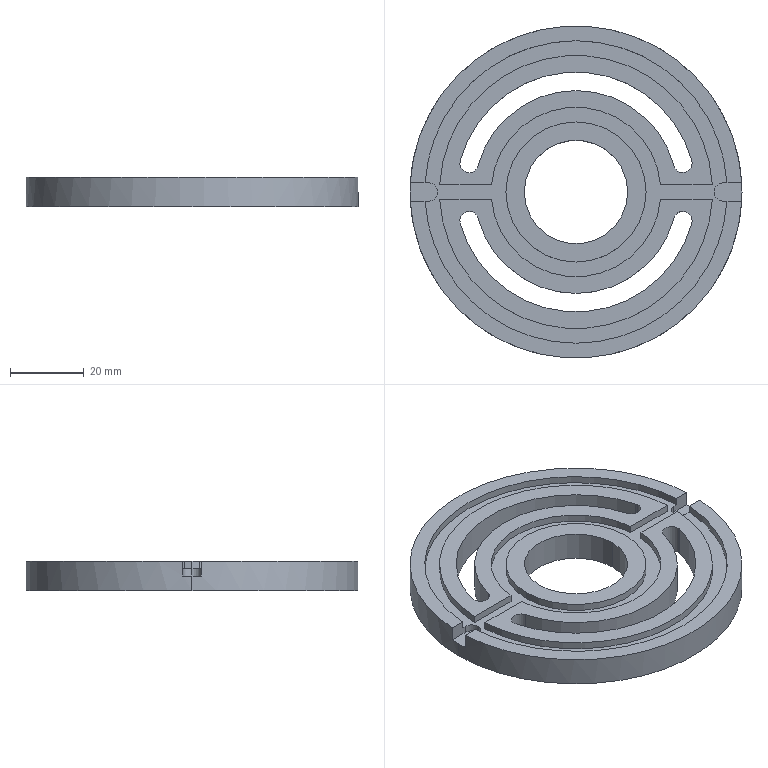Part | SolidWorks | features ICE 4, Extrusion 1 | 1 solid | 42 faces | box 90 x 90 x 8 mm | volume 35911 mm3 | cylinder 25 | plane 17 | commonest cylinder face diameters 5 x9 28 x2 38 x2 46 x2 55 x2 65 x2
STEP:
#1=CARTESIAN_POINT('',(-37.5,0.,4.));
#2=VERTEX_POINT('',#1);
#3=CARTESIAN_POINT('',(-40.,2.5,4.));
#4=VERTEX_POINT('',#3);
#5=CARTESIAN_POINT('',(-40.,0.,4.));
#6=DIRECTION('',(0.,0.,1.));
#7=DIRECTION('',(1.,0.,0.));
#8=AXIS2_PLACEMENT_3D('',#5,#6,#7);
#9=CIRCLE('',#8,2.5);
#10=EDGE_CURVE('',#2,#4,#9,.T.);
#11=ORIENTED_EDGE('',*,*,#10,.F.);
#12=CARTESIAN_POINT('',(-37.5,0.,6.));
#13=VERTEX_POINT('',#12);
#14=CARTESIAN_POINT('',(-37.5,0.,4.));
#15=DIRECTION('',(0.,0.,1.));
#16=VECTOR('',#15,1000.);
#17=LINE('',#14,#16);
#18=EDGE_CURVE('',#2,#13,#17,.T.);
#19=ORIENTED_EDGE('',*,*,#18,.T.);
#20=CARTESIAN_POINT('',(-40.,2.5,6.));
#21=VERTEX_POINT('',#20);
#22=CARTESIAN_POINT('',(-40.,0.,6.));
#23=DIRECTION('',(0.,0.,1.));
#24=DIRECTION('',(1.,0.,0.));
#25=AXIS2_PLACEMENT_3D('',#22,#23,#24);
#26=CIRCLE('',#25,2.5);
#27=EDGE_CURVE('',#13,#21,#26,.T.);
#28=ORIENTED_EDGE('',*,*,#27,.T.);
#29=CARTESIAN_POINT('',(-40.,2.5,4.));
#30=DIRECTION('',(0.,0.,1.));
#31=VECTOR('',#30,1000.);
#32=LINE('',#29,#31);
#33=EDGE_CURVE('',#4,#21,#32,.T.);
#34=ORIENTED_EDGE('',*,*,#33,.F.);
#35=EDGE_LOOP('',(#11,#19,#28,#34));
#36=FACE_OUTER_BOUND('',#35,.T.);
#37=CARTESIAN_POINT('',(-40.,0.,4.));
#38=DIRECTION('',(0.,0.,1.));
#39=DIRECTION('',(1.,0.,0.));
#40=AXIS2_PLACEMENT_3D('',#37,#38,#39);
#41=CYLINDRICAL_SURFACE('',#40,2.5);
#42=ADVANCED_FACE('',(#36),#41,.F.);
#43=CARTESIAN_POINT('',(31.478,7.765,0.));
#44=VERTEX_POINT('',#43);
#45=CARTESIAN_POINT('',(31.393,8.412,0.));
#46=VERTEX_POINT('',#45);
#47=CARTESIAN_POINT('',(28.978,7.765,0.));
#48=DIRECTION('',(0.,0.,1.));
#49=DIRECTION('',(1.,0.,0.));
#50=AXIS2_PLACEMENT_3D('',#47,#48,#49);
#51=CIRCLE('',#50,2.5);
#52=EDGE_CURVE('',#44,#46,#51,.T.);
#53=ORIENTED_EDGE('',*,*,#52,.F.);
#54=CARTESIAN_POINT('',(31.478,7.765,8.));
#55=VERTEX_POINT('',#54);
#56=CARTESIAN_POINT('',(31.478,7.765,6.));
#57=DIRECTION('',(0.,0.,1.));
#58=VECTOR('',#57,1000.);
#59=LINE('',#56,#58);
#60=EDGE_CURVE('',#44,#55,#59,.T.);
#61=ORIENTED_EDGE('',*,*,#60,.T.);
#62=CARTESIAN_POINT('',(31.393,8.412,8.));
#63=VERTEX_POINT('',#62);
#64=CARTESIAN_POINT('',(28.978,7.765,8.));
#65=DIRECTION('',(0.,0.,1.));
#66=DIRECTION('',(1.,0.,0.));
#67=AXIS2_PLACEMENT_3D('',#64,#65,#66);
#68=CIRCLE('',#67,2.5);
#69=EDGE_CURVE('',#55,#63,#68,.T.);
#70=ORIENTED_EDGE('',*,*,#69,.T.);
#71=CARTESIAN_POINT('',(31.393,8.412,6.));
#72=DIRECTION('',(0.,0.,1.));
#73=VECTOR('',#72,1000.);
#74=LINE('',#71,#73);
#75=EDGE_CURVE('',#46,#63,#74,.T.);
#76=ORIENTED_EDGE('',*,*,#75,.F.);
#77=EDGE_LOOP('',(#53,#61,#70,#76));
#78=FACE_OUTER_BOUND('',#77,.T.);
#79=CARTESIAN_POINT('',(28.978,7.765,6.));
#80=DIRECTION('',(0.,0.,1.));
#81=DIRECTION('',(1.,0.,0.));
#82=AXIS2_PLACEMENT_3D('',#79,#80,#81);
#83=CYLINDRICAL_SURFACE('',#82,2.5);
#84=ADVANCED_FACE('',(#78),#83,.F.);
#85=CARTESIAN_POINT('',(19.,0.,6.));
#86=VERTEX_POINT('',#85);
#87=CARTESIAN_POINT('',(-19.,0.,6.));
#88=VERTEX_POINT('',#87);
#89=CARTESIAN_POINT('',(0.,0.,6.));
#90=DIRECTION('',(0.,0.,1.));
#91=DIRECTION('',(1.,0.,0.));
#92=AXIS2_PLACEMENT_3D('',#89,#90,#91);
#93=CIRCLE('',#92,19.);
#94=EDGE_CURVE('',#86,#88,#93,.T.);
#95=ORIENTED_EDGE('',*,*,#94,.T.);
#96=CARTESIAN_POINT('',(-19.,0.,8.));
#97=VERTEX_POINT('',#96);
#98=CARTESIAN_POINT('',(-19.,0.,6.));
#99=DIRECTION('',(0.,0.,1.));
#100=VECTOR('',#99,1000.);
#101=LINE('',#98,#100);
#102=EDGE_CURVE('',#88,#97,#101,.T.);
#103=ORIENTED_EDGE('',*,*,#102,.T.);
#104=CARTESIAN_POINT('',(19.,0.,8.));
#105=VERTEX_POINT('',#104);
#106=CARTESIAN_POINT('',(0.,0.,8.));
#107=DIRECTION('',(0.,0.,1.));
#108=DIRECTION('',(1.,0.,0.));
#109=AXIS2_PLACEMENT_3D('',#106,#107,#108);
#110=CIRCLE('',#109,19.);
#111=EDGE_CURVE('',#105,#97,#110,.T.);
#112=ORIENTED_EDGE('',*,*,#111,.F.);
#113=CARTESIAN_POINT('',(19.,0.,6.));
#114=DIRECTION('',(0.,0.,1.));
#115=VECTOR('',#114,1000.);
#116=LINE('',#113,#115);
#117=EDGE_CURVE('',#86,#105,#116,.T.);
#118=ORIENTED_EDGE('',*,*,#117,.F.);
#119=EDGE_LOOP('',(#95,#103,#112,#118));
#120=FACE_OUTER_BOUND('',#119,.T.);
#121=CARTESIAN_POINT('',(0.,0.,6.));
#122=DIRECTION('',(0.,0.,1.));
#123=DIRECTION('',(1.,0.,0.));
#124=AXIS2_PLACEMENT_3D('',#121,#122,#123);
#125=CYLINDRICAL_SURFACE('',#124,19.);
#126=ADVANCED_FACE('',(#120),#125,.T.);
#127=CARTESIAN_POINT('',(31.478,-7.765,0.));
#128=VERTEX_POINT('',#127);
#129=CARTESIAN_POINT('',(26.563,-7.118,0.));
#130=VERTEX_POINT('',#129);
#131=CARTESIAN_POINT('',(28.978,-7.765,0.));
#132=DIRECTION('',(0.,0.,1.));
#133=DIRECTION('',(1.,0.,0.));
#134=AXIS2_PLACEMENT_3D('',#131,#132,#133);
#135=CIRCLE('',#134,2.5);
#136=EDGE_CURVE('',#128,#130,#135,.T.);
#137=ORIENTED_EDGE('',*,*,#136,.F.);
#138=CARTESIAN_POINT('',(31.478,-7.765,8.));
#139=VERTEX_POINT('',#138);
#140=CARTESIAN_POINT('',(31.478,-7.765,6.));
#141=DIRECTION('',(0.,0.,1.));
#142=VECTOR('',#141,1000.);
#143=LINE('',#140,#142);
#144=EDGE_CURVE('',#128,#139,#143,.T.);
#145=ORIENTED_EDGE('',*,*,#144,.T.);
#146=CARTESIAN_POINT('',(26.563,-7.118,8.));
#147=VERTEX_POINT('',#146);
#148=CARTESIAN_POINT('',(28.978,-7.765,8.));
#149=DIRECTION('',(0.,0.,-1.));
#150=DIRECTION('',(1.,0.,0.));
#151=AXIS2_PLACEMENT_3D('',#148,#149,#150);
#152=CIRCLE('',#151,2.5);
#153=EDGE_CURVE('',#147,#139,#152,.T.);
#154=ORIENTED_EDGE('',*,*,#153,.F.);
#155=CARTESIAN_POINT('',(26.563,-7.118,6.));
#156=DIRECTION('',(0.,0.,1.));
#157=VECTOR('',#156,1000.);
#158=LINE('',#155,#157);
#159=EDGE_CURVE('',#130,#147,#158,.T.);
#160=ORIENTED_EDGE('',*,*,#159,.F.);
#161=EDGE_LOOP('',(#137,#145,#154,#160));
#162=FACE_OUTER_BOUND('',#161,.T.);
#163=CARTESIAN_POINT('',(28.978,-7.765,6.));
#164=DIRECTION('',(0.,0.,1.));
#165=DIRECTION('',(1.,0.,0.));
#166=AXIS2_PLACEMENT_3D('',#163,#164,#165);
#167=CYLINDRICAL_SURFACE('',#166,2.5);
#168=ADVANCED_FACE('',(#162),#167,.F.);
#169=CARTESIAN_POINT('',(-14.,0.,8.));
#170=VERTEX_POINT('',#169);
#171=CARTESIAN_POINT('',(14.,0.,8.));
#172=VERTEX_POINT('',#171);
#173=CARTESIAN_POINT('',(0.,0.,8.));
#174=DIRECTION('',(0.,0.,1.));
#175=DIRECTION('',(1.,0.,0.));
#176=AXIS2_PLACEMENT_3D('',#173,#174,#175);
#177=CIRCLE('',#176,14.);
#178=EDGE_CURVE('',#170,#172,#177,.T.);
#179=ORIENTED_EDGE('',*,*,#178,.T.);
#180=CARTESIAN_POINT('',(14.,0.,0.));
#181=VERTEX_POINT('',#180);
#182=CARTESIAN_POINT('',(14.,0.,8.));
#183=DIRECTION('',(0.,0.,-1.));
#184=VECTOR('',#183,1000.);
#185=LINE('',#182,#184);
#186=EDGE_CURVE('',#172,#181,#185,.T.);
#187=ORIENTED_EDGE('',*,*,#186,.T.);
#188=CARTESIAN_POINT('',(-14.,0.,0.));
#189=VERTEX_POINT('',#188);
#190=CARTESIAN_POINT('',(0.,0.,0.));
#191=DIRECTION('',(0.,0.,1.));
#192=DIRECTION('',(1.,0.,0.));
#193=AXIS2_PLACEMENT_3D('',#190,#191,#192);
#194=CIRCLE('',#193,14.);
#195=EDGE_CURVE('',#189,#181,#194,.T.);
#196=ORIENTED_EDGE('',*,*,#195,.F.);
#197=CARTESIAN_POINT('',(-14.,0.,8.));
#198=DIRECTION('',(0.,0.,-1.));
#199=VECTOR('',#198,1000.);
#200=LINE('',#197,#199);
#201=EDGE_CURVE('',#170,#189,#200,.T.);
#202=ORIENTED_EDGE('',*,*,#201,.F.);
#203=EDGE_LOOP('',(#179,#187,#196,#202));
#204=FACE_OUTER_BOUND('',#203,.T.);
#205=CARTESIAN_POINT('',(0.,0.,8.));
#206=DIRECTION('',(0.,0.,-1.));
#207=DIRECTION('',(-1.,0.,0.));
#208=AXIS2_PLACEMENT_3D('',#205,#206,#207);
#209=CYLINDRICAL_SURFACE('',#208,14.);
#210=ADVANCED_FACE('',(#204),#209,.F.);
#211=CARTESIAN_POINT('',(45.,0.,4.));
#212=VERTEX_POINT('',#211);
#213=CARTESIAN_POINT('',(44.931,2.5,4.));
#214=VERTEX_POINT('',#213);
#215=CARTESIAN_POINT('',(0.,0.,4.));
#216=DIRECTION('',(0.,0.,1.));
#217=DIRECTION('',(1.,0.,0.));
#218=AXIS2_PLACEMENT_3D('',#215,#216,#217);
#219=CIRCLE('',#218,45.);
#220=EDGE_CURVE('',#212,#214,#219,.T.);
#221=ORIENTED_EDGE('',*,*,#220,.F.);
#222=CARTESIAN_POINT('',(45.,0.,0.));
#223=VERTEX_POINT('',#222);
#224=CARTESIAN_POINT('',(45.,0.,8.));
#225=DIRECTION('',(0.,0.,-1.));
#226=VECTOR('',#225,1000.);
#227=LINE('',#224,#226);
#228=EDGE_CURVE('',#212,#223,#227,.T.);
#229=ORIENTED_EDGE('',*,*,#228,.T.);
#230=CARTESIAN_POINT('',(-45.,0.,0.));
#231=VERTEX_POINT('',#230);
#232=CARTESIAN_POINT('',(0.,0.,0.));
#233=DIRECTION('',(0.,0.,1.));
#234=DIRECTION('',(1.,0.,0.));
#235=AXIS2_PLACEMENT_3D('',#232,#233,#234);
#236=CIRCLE('',#235,45.);
#237=EDGE_CURVE('',#223,#231,#236,.T.);
#238=ORIENTED_EDGE('',*,*,#237,.T.);
#239=CARTESIAN_POINT('',(-45.,0.,4.));
#240=VERTEX_POINT('',#239);
#241=CARTESIAN_POINT('',(-45.,0.,8.));
#242=DIRECTION('',(0.,0.,-1.));
#243=VECTOR('',#242,1000.);
#244=LINE('',#241,#243);
#245=EDGE_CURVE('',#240,#231,#244,.T.);
#246=ORIENTED_EDGE('',*,*,#245,.F.);
#247=CARTESIAN_POINT('',(-44.931,2.5,4.));
#248=VERTEX_POINT('',#247);
#249=CARTESIAN_POINT('',(0.,0.,4.));
#250=DIRECTION('',(0.,0.,1.));
#251=DIRECTION('',(1.,0.,0.));
#252=AXIS2_PLACEMENT_3D('',#249,#250,#251);
#253=CIRCLE('',#252,45.);
#254=EDGE_CURVE('',#248,#240,#253,.T.);
#255=ORIENTED_EDGE('',*,*,#254,.F.);
#256=CARTESIAN_POINT('',(-44.931,2.5,8.));
#257=VERTEX_POINT('',#256);
#258=CARTESIAN_POINT('',(-44.931,2.5,8.));
#259=DIRECTION('',(0.,0.,-1.));
#260=VECTOR('',#259,1000.);
#261=LINE('',#258,#260);
#262=EDGE_CURVE('',#257,#248,#261,.T.);
#263=ORIENTED_EDGE('',*,*,#262,.F.);
#264=CARTESIAN_POINT('',(44.931,2.5,8.));
#265=VERTEX_POINT('',#264);
#266=CARTESIAN_POINT('',(0.,0.,8.));
#267=DIRECTION('',(0.,0.,1.));
#268=DIRECTION('',(1.,0.,0.));
#269=AXIS2_PLACEMENT_3D('',#266,#267,#268);
#270=CIRCLE('',#269,45.);
#271=EDGE_CURVE('',#265,#257,#270,.T.);
#272=ORIENTED_EDGE('',*,*,#271,.F.);
#273=CARTESIAN_POINT('',(44.931,2.5,8.));
#274=DIRECTION('',(0.,0.,-1.));
#275=VECTOR('',#274,1000.);
#276=LINE('',#273,#275);
#277=EDGE_CURVE('',#265,#214,#276,.T.);
#278=ORIENTED_EDGE('',*,*,#277,.T.);
#279=EDGE_LOOP('',(#221,#229,#238,#246,#255,#263,#272,#278));
#280=FACE_OUTER_BOUND('',#279,.T.);
#281=CARTESIAN_POINT('',(0.,0.,8.));
#282=DIRECTION('',(0.,0.,-1.));
#283=DIRECTION('',(-1.,0.,0.));
#284=AXIS2_PLACEMENT_3D('',#281,#282,#283);
#285=CYLINDRICAL_SURFACE('',#284,45.);
#286=ADVANCED_FACE('',(#280),#285,.T.);
#287=CARTESIAN_POINT('',(-36.946,-2.,8.));
#288=VERTEX_POINT('',#287);
#289=CARTESIAN_POINT('',(36.946,-2.,8.));
#290=VERTEX_POINT('',#289);
#291=CARTESIAN_POINT('',(0.,0.,8.));
#292=DIRECTION('',(0.,0.,1.));
#293=DIRECTION('',(1.,0.,0.));
#294=AXIS2_PLACEMENT_3D('',#291,#292,#293);
#295=CIRCLE('',#294,37.);
#296=EDGE_CURVE('',#288,#290,#295,.T.);
#297=ORIENTED_EDGE('',*,*,#296,.F.);
#298=CARTESIAN_POINT('',(-36.946,-2.,6.));
#299=VERTEX_POINT('',#298);
#300=CARTESIAN_POINT('',(-36.946,-2.,6.));
#301=DIRECTION('',(0.,0.,1.));
#302=VECTOR('',#301,1000.);
#303=LINE('',#300,#302);
#304=EDGE_CURVE('',#299,#288,#303,.T.);
#305=ORIENTED_EDGE('',*,*,#304,.F.);
#306=CARTESIAN_POINT('',(36.946,-2.,6.));
#307=VERTEX_POINT('',#306);
#308=CARTESIAN_POINT('',(0.,0.,6.));
#309=DIRECTION('',(0.,0.,1.));
#310=DIRECTION('',(1.,0.,0.));
#311=AXIS2_PLACEMENT_3D('',#308,#309,#310);
#312=CIRCLE('',#311,37.);
#313=EDGE_CURVE('',#299,#307,#312,.T.);
#314=ORIENTED_EDGE('',*,*,#313,.T.);
#315=CARTESIAN_POINT('',(36.946,-2.,6.));
#316=DIRECTION('',(0.,0.,1.));
#317=VECTOR('',#316,1000.);
#318=LINE('',#315,#317);
#319=EDGE_CURVE('',#307,#290,#318,.T.);
#320=ORIENTED_EDGE('',*,*,#319,.T.);
#321=EDGE_LOOP('',(#297,#305,#314,#320));
#322=FACE_OUTER_BOUND('',#321,.T.);
#323=CARTESIAN_POINT('',(0.,0.,6.));
#324=DIRECTION('',(0.,0.,1.));
#325=DIRECTION('',(1.,0.,0.));
#326=AXIS2_PLACEMENT_3D('',#323,#324,#325);
#327=CYLINDRICAL_SURFACE('',#326,37.);
#328=ADVANCED_FACE('',(#322),#327,.T.);
#329=CARTESIAN_POINT('',(-36.946,2.,6.));
#330=VERTEX_POINT('',#329);
#331=CARTESIAN_POINT('',(-36.946,2.,8.));
#332=VERTEX_POINT('',#331);
#333=CARTESIAN_POINT('',(-36.946,2.,6.));
#334=DIRECTION('',(0.,0.,1.));
#335=VECTOR('',#334,1000.);
#336=LINE('',#333,#335);
#337=EDGE_CURVE('',#330,#332,#336,.T.);
#338=ORIENTED_EDGE('',*,*,#337,.T.);
#339=CARTESIAN_POINT('',(36.946,2.,8.));
#340=VERTEX_POINT('',#339);
#341=CARTESIAN_POINT('',(0.,0.,8.));
#342=DIRECTION('',(0.,0.,1.));
#343=DIRECTION('',(1.,0.,0.));
#344=AXIS2_PLACEMENT_3D('',#341,#342,#343);
#345=CIRCLE('',#344,37.);
#346=EDGE_CURVE('',#340,#332,#345,.T.);
#347=ORIENTED_EDGE('',*,*,#346,.F.);
#348=CARTESIAN_POINT('',(36.946,2.,6.));
#349=VERTEX_POINT('',#348);
#350=CARTESIAN_POINT('',(36.946,2.,6.));
#351=DIRECTION('',(0.,0.,1.));
#352=VECTOR('',#351,1000.);
#353=LINE('',#350,#352);
#354=EDGE_CURVE('',#349,#340,#353,.T.);
#355=ORIENTED_EDGE('',*,*,#354,.F.);
#356=CARTESIAN_POINT('',(0.,0.,6.));
#357=DIRECTION('',(0.,0.,1.));
#358=DIRECTION('',(1.,0.,0.));
#359=AXIS2_PLACEMENT_3D('',#356,#357,#358);
#360=CIRCLE('',#359,37.);
#361=EDGE_CURVE('',#349,#330,#360,.T.);
#362=ORIENTED_EDGE('',*,*,#361,.T.);
#363=EDGE_LOOP('',(#338,#347,#355,#362));
#364=FACE_OUTER_BOUND('',#363,.T.);
#365=CARTESIAN_POINT('',(0.,0.,6.));
#366=DIRECTION('',(0.,0.,1.));
#367=DIRECTION('',(1.,0.,0.));
#368=AXIS2_PLACEMENT_3D('',#365,#366,#367);
#369=CYLINDRICAL_SURFACE('',#368,37.);
#370=ADVANCED_FACE('',(#364),#369,.T.);
#371=CARTESIAN_POINT('',(31.393,-8.412,8.));
#372=VERTEX_POINT('',#371);
#373=CARTESIAN_POINT('',(-31.393,-8.412,8.));
#374=VERTEX_POINT('',#373);
#375=CARTESIAN_POINT('',(0.,0.,8.));
#376=DIRECTION('',(0.,0.,-1.));
#377=DIRECTION('',(1.,0.,0.));
#378=AXIS2_PLACEMENT_3D('',#375,#376,#377);
#379=CIRCLE('',#378,32.5);
#380=EDGE_CURVE('',#372,#374,#379,.T.);
#381=ORIENTED_EDGE('',*,*,#380,.T.);
#382=CARTESIAN_POINT('',(-26.563,-7.118,8.));
#383=VERTEX_POINT('',#382);
#384=CARTESIAN_POINT('',(-28.978,-7.765,8.));
#385=DIRECTION('',(0.,0.,-1.));
#386=DIRECTION('',(1.,0.,0.));
#387=AXIS2_PLACEMENT_3D('',#384,#385,#386);
#388=CIRCLE('',#387,2.5);
#389=EDGE_CURVE('',#374,#383,#388,.T.);
#390=ORIENTED_EDGE('',*,*,#389,.T.);
#391=CARTESIAN_POINT('',(0.,0.,8.));
#392=DIRECTION('',(0.,0.,-1.));
#393=DIRECTION('',(1.,0.,0.));
#394=AXIS2_PLACEMENT_3D('',#391,#392,#393);
#395=CIRCLE('',#394,27.5);
#396=EDGE_CURVE('',#147,#383,#395,.T.);
#397=ORIENTED_EDGE('',*,*,#396,.F.);
#398=ORIENTED_EDGE('',*,*,#153,.T.);
#399=CARTESIAN_POINT('',(28.978,-7.765,8.));
#400=DIRECTION('',(0.,0.,-1.));
#401=DIRECTION('',(1.,0.,0.));
#402=AXIS2_PLACEMENT_3D('',#399,#400,#401);
#403=CIRCLE('',#402,2.5);
#404=EDGE_CURVE('',#139,#372,#403,.T.);
#405=ORIENTED_EDGE('',*,*,#404,.T.);
#406=EDGE_LOOP('',(#381,#390,#397,#398,#405));
#407=FACE_BOUND('',#406,.T.);
#408=CARTESIAN_POINT('',(-22.913,-2.,8.));
#409=VERTEX_POINT('',#408);
#410=CARTESIAN_POINT('',(22.913,-2.,8.));
#411=VERTEX_POINT('',#410);
#412=CARTESIAN_POINT('',(0.,0.,8.));
#413=DIRECTION('',(0.,0.,1.));
#414=DIRECTION('',(1.,0.,0.));
#415=AXIS2_PLACEMENT_3D('',#412,#413,#414);
#416=CIRCLE('',#415,23.);
#417=EDGE_CURVE('',#409,#411,#416,.T.);
#418=ORIENTED_EDGE('',*,*,#417,.F.);
#419=CARTESIAN_POINT('',(0.,-2.,8.));
#420=DIRECTION('',(-1.,0.,0.));
#421=VECTOR('',#420,1000.);
#422=LINE('',#419,#421);
#423=EDGE_CURVE('',#409,#288,#422,.T.);
#424=ORIENTED_EDGE('',*,*,#423,.T.);
#425=ORIENTED_EDGE('',*,*,#296,.T.);
#426=CARTESIAN_POINT('',(0.,-2.,8.));
#427=DIRECTION('',(-1.,0.,0.));
#428=VECTOR('',#427,1000.);
#429=LINE('',#426,#428);
#430=EDGE_CURVE('',#290,#411,#429,.T.);
#431=ORIENTED_EDGE('',*,*,#430,.T.);
#432=EDGE_LOOP('',(#418,#424,#425,#431));
#433=FACE_OUTER_BOUND('',#432,.T.);
#434=CARTESIAN_POINT('',(0.,0.,8.));
#435=DIRECTION('',(0.,0.,1.));
#436=DIRECTION('',(1.,0.,0.));
#437=AXIS2_PLACEMENT_3D('',#434,#435,#436);
#438=PLANE('',#437);
#439=ADVANCED_FACE('',(#407,#433),#438,.T.);
#440=CARTESIAN_POINT('',(-22.913,2.,8.));
#441=VERTEX_POINT('',#440);
#442=CARTESIAN_POINT('',(0.,2.,8.));
#443=DIRECTION('',(-1.,0.,0.));
#444=VECTOR('',#443,1000.);
#445=LINE('',#442,#444);
#446=EDGE_CURVE('',#441,#332,#445,.T.);
#447=ORIENTED_EDGE('',*,*,#446,.F.);
#448=CARTESIAN_POINT('',(22.913,2.,8.));
#449=VERTEX_POINT('',#448);
#450=CARTESIAN_POINT('',(0.,0.,8.));
#451=DIRECTION('',(0.,0.,1.));
#452=DIRECTION('',(1.,0.,0.));
#453=AXIS2_PLACEMENT_3D('',#450,#451,#452);
#454=CIRCLE('',#453,23.);
#455=EDGE_CURVE('',#449,#441,#454,.T.);
#456=ORIENTED_EDGE('',*,*,#455,.F.);
#457=CARTESIAN_POINT('',(0.,2.,8.));
#458=DIRECTION('',(-1.,0.,0.));
#459=VECTOR('',#458,1000.);
#460=LINE('',#457,#459);
#461=EDGE_CURVE('',#340,#449,#460,.T.);
#462=ORIENTED_EDGE('',*,*,#461,.F.);
#463=ORIENTED_EDGE('',*,*,#346,.T.);
#464=EDGE_LOOP('',(#447,#456,#462,#463));
#465=FACE_OUTER_BOUND('',#464,.T.);
#466=CARTESIAN_POINT('',(-31.393,8.412,8.));
#467=VERTEX_POINT('',#466);
#468=CARTESIAN_POINT('',(0.,0.,8.));
#469=DIRECTION('',(0.,0.,1.));
#470=DIRECTION('',(1.,0.,0.));
#471=AXIS2_PLACEMENT_3D('',#468,#469,#470);
#472=CIRCLE('',#471,32.5);
#473=EDGE_CURVE('',#63,#467,#472,.T.);
#474=ORIENTED_EDGE('',*,*,#473,.F.);
#475=ORIENTED_EDGE('',*,*,#69,.F.);
#476=CARTESIAN_POINT('',(26.563,7.118,8.));
#477=VERTEX_POINT('',#476);
#478=CARTESIAN_POINT('',(28.978,7.765,8.));
#479=DIRECTION('',(0.,0.,1.));
#480=DIRECTION('',(1.,0.,0.));
#481=AXIS2_PLACEMENT_3D('',#478,#479,#480);
#482=CIRCLE('',#481,2.5);
#483=EDGE_CURVE('',#477,#55,#482,.T.);
#484=ORIENTED_EDGE('',*,*,#483,.F.);
#485=CARTESIAN_POINT('',(-26.563,7.118,8.));
#486=VERTEX_POINT('',#485);
#487=CARTESIAN_POINT('',(0.,0.,8.));
#488=DIRECTION('',(0.,0.,1.));
#489=DIRECTION('',(1.,0.,0.));
#490=AXIS2_PLACEMENT_3D('',#487,#488,#489);
#491=CIRCLE('',#490,27.5);
#492=EDGE_CURVE('',#477,#486,#491,.T.);
#493=ORIENTED_EDGE('',*,*,#492,.T.);
#494=CARTESIAN_POINT('',(-28.978,7.765,8.));
#495=DIRECTION('',(0.,0.,1.));
#496=DIRECTION('',(1.,0.,0.));
#497=AXIS2_PLACEMENT_3D('',#494,#495,#496);
#498=CIRCLE('',#497,2.5);
#499=EDGE_CURVE('',#467,#486,#498,.T.);
#500=ORIENTED_EDGE('',*,*,#499,.F.);
#501=EDGE_LOOP('',(#474,#475,#484,#493,#500));
#502=FACE_BOUND('',#501,.T.);
#503=CARTESIAN_POINT('',(0.,0.,8.));
#504=DIRECTION('',(0.,0.,1.));
#505=DIRECTION('',(1.,0.,0.));
#506=AXIS2_PLACEMENT_3D('',#503,#504,#505);
#507=PLANE('',#506);
#508=ADVANCED_FACE('',(#465,#502),#507,.T.);
#509=CARTESIAN_POINT('',(-22.913,-2.,6.));
#510=VERTEX_POINT('',#509);
#511=CARTESIAN_POINT('',(-22.913,-2.,6.));
#512=DIRECTION('',(0.,0.,1.));
#513=VECTOR('',#512,1000.);
#514=LINE('',#511,#513);
#515=EDGE_CURVE('',#510,#409,#514,.T.);
#516=ORIENTED_EDGE('',*,*,#515,.T.);
#517=ORIENTED_EDGE('',*,*,#417,.T.);
#518=CARTESIAN_POINT('',(22.913,-2.,6.));
#519=VERTEX_POINT('',#518);
#520=CARTESIAN_POINT('',(22.913,-2.,6.));
#521=DIRECTION('',(0.,0.,1.));
#522=VECTOR('',#521,1000.);
#523=LINE('',#520,#522);
#524=EDGE_CURVE('',#519,#411,#523,.T.);
#525=ORIENTED_EDGE('',*,*,#524,.F.);
#526=CARTESIAN_POINT('',(0.,0.,6.));
#527=DIRECTION('',(0.,0.,1.));
#528=DIRECTION('',(1.,0.,0.));
#529=AXIS2_PLACEMENT_3D('',#526,#527,#528);
#530=CIRCLE('',#529,23.);
#531=EDGE_CURVE('',#510,#519,#530,.T.);
#532=ORIENTED_EDGE('',*,*,#531,.F.);
#533=EDGE_LOOP('',(#516,#517,#525,#532));
#534=FACE_OUTER_BOUND('',#533,.T.);
#535=CARTESIAN_POINT('',(0.,0.,6.));
#536=DIRECTION('',(0.,0.,1.));
#537=DIRECTION('',(1.,0.,0.));
#538=AXIS2_PLACEMENT_3D('',#535,#536,#537);
#539=CYLINDRICAL_SURFACE('',#538,23.);
#540=ADVANCED_FACE('',(#534),#539,.F.);
#541=ORIENTED_EDGE('',*,*,#455,.T.);
#542=CARTESIAN_POINT('',(-22.913,2.,6.));
#543=VERTEX_POINT('',#542);
#544=CARTESIAN_POINT('',(-22.913,2.,6.));
#545=DIRECTION('',(0.,0.,1.));
#546=VECTOR('',#545,1000.);
#547=LINE('',#544,#546);
#548=EDGE_CURVE('',#543,#441,#547,.T.);
#549=ORIENTED_EDGE('',*,*,#548,.F.);
#550=CARTESIAN_POINT('',(22.913,2.,6.));
#551=VERTEX_POINT('',#550);
#552=CARTESIAN_POINT('',(0.,0.,6.));
#553=DIRECTION('',(0.,0.,1.));
#554=DIRECTION('',(1.,0.,0.));
#555=AXIS2_PLACEMENT_3D('',#552,#553,#554);
#556=CIRCLE('',#555,23.);
#557=EDGE_CURVE('',#551,#543,#556,.T.);
#558=ORIENTED_EDGE('',*,*,#557,.F.);
#559=CARTESIAN_POINT('',(22.913,2.,6.));
#560=DIRECTION('',(0.,0.,1.));
#561=VECTOR('',#560,1000.);
#562=LINE('',#559,#561);
#563=EDGE_CURVE('',#551,#449,#562,.T.);
#564=ORIENTED_EDGE('',*,*,#563,.T.);
#565=EDGE_LOOP('',(#541,#549,#558,#564));
#566=FACE_OUTER_BOUND('',#565,.T.);
#567=CARTESIAN_POINT('',(0.,0.,6.));
#568=DIRECTION('',(0.,0.,1.));
#569=DIRECTION('',(1.,0.,0.));
#570=AXIS2_PLACEMENT_3D('',#567,#568,#569);
#571=CYLINDRICAL_SURFACE('',#570,23.);
#572=ADVANCED_FACE('',(#566),#571,.F.);
#573=ORIENTED_EDGE('',*,*,#271,.T.);
#574=CARTESIAN_POINT('',(-40.924,2.5,8.));
#575=VERTEX_POINT('',#574);
#576=CARTESIAN_POINT('',(0.,2.5,8.));
#577=DIRECTION('',(1.,0.,0.));
#578=VECTOR('',#577,1000.);
#579=LINE('',#576,#578);
#580=EDGE_CURVE('',#257,#575,#579,.T.);
#581=ORIENTED_EDGE('',*,*,#580,.T.);
#582=CARTESIAN_POINT('',(40.924,2.5,8.));
#583=VERTEX_POINT('',#582);
#584=CARTESIAN_POINT('',(0.,0.,8.));
#585=DIRECTION('',(0.,0.,1.));
#586=DIRECTION('',(1.,0.,0.));
#587=AXIS2_PLACEMENT_3D('',#584,#585,#586);
#588=CIRCLE('',#587,41.);
#589=EDGE_CURVE('',#583,#575,#588,.T.);
#590=ORIENTED_EDGE('',*,*,#589,.F.);
#591=CARTESIAN_POINT('',(0.,2.5,8.));
#592=DIRECTION('',(-1.,0.,0.));
#593=VECTOR('',#592,1000.);
#594=LINE('',#591,#593);
#595=EDGE_CURVE('',#265,#583,#594,.T.);
#596=ORIENTED_EDGE('',*,*,#595,.F.);
#597=EDGE_LOOP('',(#573,#581,#590,#596));
#598=FACE_OUTER_BOUND('',#597,.T.);
#599=CARTESIAN_POINT('',(0.,0.,8.));
#600=DIRECTION('',(0.,0.,1.));
#601=DIRECTION('',(1.,0.,0.));
#602=AXIS2_PLACEMENT_3D('',#599,#600,#601);
#603=PLANE('',#602);
#604=ADVANCED_FACE('',(#598),#603,.T.);
#605=CARTESIAN_POINT('',(-40.924,2.5,6.));
#606=VERTEX_POINT('',#605);
#607=CARTESIAN_POINT('',(-40.924,2.5,6.));
#608=DIRECTION('',(0.,0.,1.));
#609=VECTOR('',#608,1000.);
#610=LINE('',#607,#609);
#611=EDGE_CURVE('',#606,#575,#610,.T.);
#612=ORIENTED_EDGE('',*,*,#611,.F.);
#613=CARTESIAN_POINT('',(40.924,2.5,6.));
#614=VERTEX_POINT('',#613);
#615=CARTESIAN_POINT('',(0.,0.,6.));
#616=DIRECTION('',(0.,0.,1.));
#617=DIRECTION('',(1.,0.,0.));
#618=AXIS2_PLACEMENT_3D('',#615,#616,#617);
#619=CIRCLE('',#618,41.);
#620=EDGE_CURVE('',#614,#606,#619,.T.);
#621=ORIENTED_EDGE('',*,*,#620,.F.);
#622=CARTESIAN_POINT('',(40.924,2.5,6.));
#623=DIRECTION('',(0.,0.,1.));
#624=VECTOR('',#623,1000.);
#625=LINE('',#622,#624);
#626=EDGE_CURVE('',#614,#583,#625,.T.);
#627=ORIENTED_EDGE('',*,*,#626,.T.);
#628=ORIENTED_EDGE('',*,*,#589,.T.);
#629=EDGE_LOOP('',(#612,#621,#627,#628));
#630=FACE_OUTER_BOUND('',#629,.T.);
#631=CARTESIAN_POINT('',(0.,0.,6.));
#632=DIRECTION('',(0.,0.,1.));
#633=DIRECTION('',(1.,0.,0.));
#634=AXIS2_PLACEMENT_3D('',#631,#632,#633);
#635=CYLINDRICAL_SURFACE('',#634,41.);
#636=ADVANCED_FACE('',(#630),#635,.F.);
#637=ORIENTED_EDGE('',*,*,#178,.F.);
#638=CARTESIAN_POINT('',(0.,0.,8.));
#639=DIRECTION('',(0.,0.,1.));
#640=DIRECTION('',(1.,0.,0.));
#641=AXIS2_PLACEMENT_3D('',#638,#639,#640);
#642=CIRCLE('',#641,14.);
#643=EDGE_CURVE('',#172,#170,#642,.T.);
#644=ORIENTED_EDGE('',*,*,#643,.F.);
#645=EDGE_LOOP('',(#637,#644));
#646=FACE_BOUND('',#645,.T.);
#647=ORIENTED_EDGE('',*,*,#111,.T.);
#648=CARTESIAN_POINT('',(0.,0.,8.));
#649=DIRECTION('',(0.,0.,1.));
#650=DIRECTION('',(1.,0.,0.));
#651=AXIS2_PLACEMENT_3D('',#648,#649,#650);
#652=CIRCLE('',#651,19.);
#653=EDGE_CURVE('',#97,#105,#652,.T.);
#654=ORIENTED_EDGE('',*,*,#653,.T.);
#655=EDGE_LOOP('',(#647,#654));
#656=FACE_OUTER_BOUND('',#655,.T.);
#657=CARTESIAN_POINT('',(0.,0.,8.));
#658=DIRECTION('',(0.,0.,1.));
#659=DIRECTION('',(1.,0.,0.));
#660=AXIS2_PLACEMENT_3D('',#657,#658,#659);
#661=PLANE('',#660);
#662=ADVANCED_FACE('',(#646,#656),#661,.T.);
#663=CARTESIAN_POINT('',(-44.931,-2.5,8.));
#664=VERTEX_POINT('',#663);
#665=CARTESIAN_POINT('',(-40.924,-2.5,8.));
#666=VERTEX_POINT('',#665);
#667=CARTESIAN_POINT('',(0.,-2.5,8.));
#668=DIRECTION('',(1.,0.,0.));
#669=VECTOR('',#668,1000.);
#670=LINE('',#667,#669);
#671=EDGE_CURVE('',#664,#666,#670,.T.);
#672=ORIENTED_EDGE('',*,*,#671,.F.);
#673=CARTESIAN_POINT('',(44.931,-2.5,8.));
#674=VERTEX_POINT('',#673);
#675=CARTESIAN_POINT('',(0.,0.,8.));
#676=DIRECTION('',(0.,0.,1.));
#677=DIRECTION('',(1.,0.,0.));
#678=AXIS2_PLACEMENT_3D('',#675,#676,#677);
#679=CIRCLE('',#678,45.);
#680=EDGE_CURVE('',#664,#674,#679,.T.);
#681=ORIENTED_EDGE('',*,*,#680,.T.);
#682=CARTESIAN_POINT('',(40.924,-2.5,8.));
#683=VERTEX_POINT('',#682);
#684=CARTESIAN_POINT('',(0.,-2.5,8.));
#685=DIRECTION('',(-1.,0.,0.));
#686=VECTOR('',#685,1000.);
#687=LINE('',#684,#686);
#688=EDGE_CURVE('',#674,#683,#687,.T.);
#689=ORIENTED_EDGE('',*,*,#688,.T.);
#690=CARTESIAN_POINT('',(0.,0.,8.));
#691=DIRECTION('',(0.,0.,1.));
#692=DIRECTION('',(1.,0.,0.));
#693=AXIS2_PLACEMENT_3D('',#690,#691,#692);
#694=CIRCLE('',#693,41.);
#695=EDGE_CURVE('',#666,#683,#694,.T.);
#696=ORIENTED_EDGE('',*,*,#695,.F.);
#697=EDGE_LOOP('',(#672,#681,#689,#696));
#698=FACE_OUTER_BOUND('',#697,.T.);
#699=CARTESIAN_POINT('',(0.,0.,8.));
#700=DIRECTION('',(0.,0.,1.));
#701=DIRECTION('',(1.,0.,0.));
#702=AXIS2_PLACEMENT_3D('',#699,#700,#701);
#703=PLANE('',#702);
#704=ADVANCED_FACE('',(#698),#703,.T.);
#705=CARTESIAN_POINT('',(-26.563,7.118,0.));
#706=VERTEX_POINT('',#705);
#707=CARTESIAN_POINT('',(26.563,7.118,0.));
#708=VERTEX_POINT('',#707);
#709=CARTESIAN_POINT('',(0.,0.,0.));
#710=DIRECTION('',(0.,0.,-1.));
#711=DIRECTION('',(1.,0.,0.));
#712=AXIS2_PLACEMENT_3D('',#709,#710,#711);
#713=CIRCLE('',#712,27.5);
#714=EDGE_CURVE('',#706,#708,#713,.T.);
#715=ORIENTED_EDGE('',*,*,#714,.T.);
#716=CARTESIAN_POINT('',(28.978,7.765,0.));
#717=DIRECTION('',(0.,0.,1.));
#718=DIRECTION('',(1.,0.,0.));
#719=AXIS2_PLACEMENT_3D('',#716,#717,#718);
#720=CIRCLE('',#719,2.5);
#721=EDGE_CURVE('',#708,#44,#720,.T.);
#722=ORIENTED_EDGE('',*,*,#721,.T.);
#723=ORIENTED_EDGE('',*,*,#52,.T.);
#724=CARTESIAN_POINT('',(-31.393,8.412,0.));
#725=VERTEX_POINT('',#724);
#726=CARTESIAN_POINT('',(0.,0.,0.));
#727=DIRECTION('',(0.,0.,1.));
#728=DIRECTION('',(1.,0.,0.));
#729=AXIS2_PLACEMENT_3D('',#726,#727,#728);
#730=CIRCLE('',#729,32.5);
#731=EDGE_CURVE('',#46,#725,#730,.T.);
#732=ORIENTED_EDGE('',*,*,#731,.T.);
#733=CARTESIAN_POINT('',(-28.978,7.765,0.));
#734=DIRECTION('',(0.,0.,1.));
#735=DIRECTION('',(1.,0.,0.));
#736=AXIS2_PLACEMENT_3D('',#733,#734,#735);
#737=CIRCLE('',#736,2.5);
#738=EDGE_CURVE('',#725,#706,#737,.T.);
#739=ORIENTED_EDGE('',*,*,#738,.T.);
#740=EDGE_LOOP('',(#715,#722,#723,#732,#739));
#741=FACE_BOUND('',#740,.T.);
#742=CARTESIAN_POINT('',(31.393,-8.412,0.));
#743=VERTEX_POINT('',#742);
#744=CARTESIAN_POINT('',(28.978,-7.765,0.));
#745=DIRECTION('',(0.,0.,1.));
#746=DIRECTION('',(1.,0.,0.));
#747=AXIS2_PLACEMENT_3D('',#744,#745,#746);
#748=CIRCLE('',#747,2.5);
#749=EDGE_CURVE('',#743,#128,#748,.T.);
#750=ORIENTED_EDGE('',*,*,#749,.T.);
#751=ORIENTED_EDGE('',*,*,#136,.T.);
#752=CARTESIAN_POINT('',(-26.563,-7.118,0.));
#753=VERTEX_POINT('',#752);
#754=CARTESIAN_POINT('',(0.,0.,0.));
#755=DIRECTION('',(0.,0.,-1.));
#756=DIRECTION('',(1.,0.,0.));
#757=AXIS2_PLACEMENT_3D('',#754,#755,#756);
#758=CIRCLE('',#757,27.5);
#759=EDGE_CURVE('',#130,#753,#758,.T.);
#760=ORIENTED_EDGE('',*,*,#759,.T.);
#761=CARTESIAN_POINT('',(-31.393,-8.412,0.));
#762=VERTEX_POINT('',#761);
#763=CARTESIAN_POINT('',(-28.978,-7.765,0.));
#764=DIRECTION('',(0.,0.,1.));
#765=DIRECTION('',(1.,0.,0.));
#766=AXIS2_PLACEMENT_3D('',#763,#764,#765);
#767=CIRCLE('',#766,2.5);
#768=EDGE_CURVE('',#753,#762,#767,.T.);
#769=ORIENTED_EDGE('',*,*,#768,.T.);
#770=CARTESIAN_POINT('',(0.,0.,0.));
#771=DIRECTION('',(0.,0.,1.));
#772=DIRECTION('',(1.,0.,0.));
#773=AXIS2_PLACEMENT_3D('',#770,#771,#772);
#774=CIRCLE('',#773,32.5);
#775=EDGE_CURVE('',#762,#743,#774,.T.);
#776=ORIENTED_EDGE('',*,*,#775,.T.);
#777=EDGE_LOOP('',(#750,#751,#760,#769,#776));
#778=FACE_BOUND('',#777,.T.);
#779=CARTESIAN_POINT('',(0.,0.,0.));
#780=DIRECTION('',(0.,0.,1.));
#781=DIRECTION('',(1.,0.,0.));
#782=AXIS2_PLACEMENT_3D('',#779,#780,#781);
#783=CIRCLE('',#782,45.);
#784=EDGE_CURVE('',#231,#223,#783,.T.);
#785=ORIENTED_EDGE('',*,*,#784,.F.);
#786=ORIENTED_EDGE('',*,*,#237,.F.);
#787=EDGE_LOOP('',(#785,#786));
#788=FACE_OUTER_BOUND('',#787,.T.);
#789=ORIENTED_EDGE('',*,*,#195,.T.);
#790=CARTESIAN_POINT('',(0.,0.,0.));
#791=DIRECTION('',(0.,0.,1.));
#792=DIRECTION('',(1.,0.,0.));
#793=AXIS2_PLACEMENT_3D('',#790,#791,#792);
#794=CIRCLE('',#793,14.);
#795=EDGE_CURVE('',#181,#189,#794,.T.);
#796=ORIENTED_EDGE('',*,*,#795,.T.);
#797=EDGE_LOOP('',(#789,#796));
#798=FACE_BOUND('',#797,.T.);
#799=CARTESIAN_POINT('',(0.,0.,0.));
#800=DIRECTION('',(0.,0.,1.));
#801=DIRECTION('',(1.,0.,0.));
#802=AXIS2_PLACEMENT_3D('',#799,#800,#801);
#803=PLANE('',#802);
#804=ADVANCED_FACE('',(#741,#778,#788,#798),#803,.F.);
#805=ORIENTED_EDGE('',*,*,#228,.F.);
#806=CARTESIAN_POINT('',(44.931,-2.5,4.));
#807=VERTEX_POINT('',#806);
#808=CARTESIAN_POINT('',(0.,0.,4.));
#809=DIRECTION('',(0.,0.,1.));
#810=DIRECTION('',(1.,0.,0.));
#811=AXIS2_PLACEMENT_3D('',#808,#809,#810);
#812=CIRCLE('',#811,45.);
#813=EDGE_CURVE('',#807,#212,#812,.T.);
#814=ORIENTED_EDGE('',*,*,#813,.F.);
#815=CARTESIAN_POINT('',(44.931,-2.5,8.));
#816=DIRECTION('',(0.,0.,-1.));
#817=VECTOR('',#816,1000.);
#818=LINE('',#815,#817);
#819=EDGE_CURVE('',#674,#807,#818,.T.);
#820=ORIENTED_EDGE('',*,*,#819,.F.);
#821=ORIENTED_EDGE('',*,*,#680,.F.);
#822=CARTESIAN_POINT('',(-44.931,-2.5,4.));
#823=VERTEX_POINT('',#822);
#824=CARTESIAN_POINT('',(-44.931,-2.5,8.));
#825=DIRECTION('',(0.,0.,-1.));
#826=VECTOR('',#825,1000.);
#827=LINE('',#824,#826);
#828=EDGE_CURVE('',#664,#823,#827,.T.);
#829=ORIENTED_EDGE('',*,*,#828,.T.);
#830=CARTESIAN_POINT('',(0.,0.,4.));
#831=DIRECTION('',(0.,0.,1.));
#832=DIRECTION('',(1.,0.,0.));
#833=AXIS2_PLACEMENT_3D('',#830,#831,#832);
#834=CIRCLE('',#833,45.);
#835=EDGE_CURVE('',#240,#823,#834,.T.);
#836=ORIENTED_EDGE('',*,*,#835,.F.);
#837=ORIENTED_EDGE('',*,*,#245,.T.);
#838=ORIENTED_EDGE('',*,*,#784,.T.);
#839=EDGE_LOOP('',(#805,#814,#820,#821,#829,#836,#837,#838));
#840=FACE_OUTER_BOUND('',#839,.T.);
#841=CARTESIAN_POINT('',(0.,0.,8.));
#842=DIRECTION('',(0.,0.,-1.));
#843=DIRECTION('',(-1.,0.,0.));
#844=AXIS2_PLACEMENT_3D('',#841,#842,#843);
#845=CYLINDRICAL_SURFACE('',#844,45.);
#846=ADVANCED_FACE('',(#840),#845,.T.);
#847=ORIENTED_EDGE('',*,*,#186,.F.);
#848=ORIENTED_EDGE('',*,*,#643,.T.);
#849=ORIENTED_EDGE('',*,*,#201,.T.);
#850=ORIENTED_EDGE('',*,*,#795,.F.);
#851=EDGE_LOOP('',(#847,#848,#849,#850));
#852=FACE_OUTER_BOUND('',#851,.T.);
#853=CARTESIAN_POINT('',(0.,0.,8.));
#854=DIRECTION('',(0.,0.,-1.));
#855=DIRECTION('',(-1.,0.,0.));
#856=AXIS2_PLACEMENT_3D('',#853,#854,#855);
#857=CYLINDRICAL_SURFACE('',#856,14.);
#858=ADVANCED_FACE('',(#852),#857,.F.);
#859=CARTESIAN_POINT('',(-40.924,-2.5,6.));
#860=VERTEX_POINT('',#859);
#861=CARTESIAN_POINT('',(40.924,-2.5,6.));
#862=VERTEX_POINT('',#861);
#863=CARTESIAN_POINT('',(0.,0.,6.));
#864=DIRECTION('',(0.,0.,1.));
#865=DIRECTION('',(1.,0.,0.));
#866=AXIS2_PLACEMENT_3D('',#863,#864,#865);
#867=CIRCLE('',#866,41.);
#868=EDGE_CURVE('',#860,#862,#867,.T.);
#869=ORIENTED_EDGE('',*,*,#868,.F.);
#870=CARTESIAN_POINT('',(-40.924,-2.5,6.));
#871=DIRECTION('',(0.,0.,1.));
#872=VECTOR('',#871,1000.);
#873=LINE('',#870,#872);
#874=EDGE_CURVE('',#860,#666,#873,.T.);
#875=ORIENTED_EDGE('',*,*,#874,.T.);
#876=ORIENTED_EDGE('',*,*,#695,.T.);
#877=CARTESIAN_POINT('',(40.924,-2.5,6.));
#878=DIRECTION('',(0.,0.,1.));
#879=VECTOR('',#878,1000.);
#880=LINE('',#877,#879);
#881=EDGE_CURVE('',#862,#683,#880,.T.);
#882=ORIENTED_EDGE('',*,*,#881,.F.);
#883=EDGE_LOOP('',(#869,#875,#876,#882));
#884=FACE_OUTER_BOUND('',#883,.T.);
#885=CARTESIAN_POINT('',(0.,0.,6.));
#886=DIRECTION('',(0.,0.,1.));
#887=DIRECTION('',(1.,0.,0.));
#888=AXIS2_PLACEMENT_3D('',#885,#886,#887);
#889=CYLINDRICAL_SURFACE('',#888,41.);
#890=ADVANCED_FACE('',(#884),#889,.F.);
#891=ORIENTED_EDGE('',*,*,#389,.F.);
#892=CARTESIAN_POINT('',(-31.393,-8.412,6.));
#893=DIRECTION('',(0.,0.,1.));
#894=VECTOR('',#893,1000.);
#895=LINE('',#892,#894);
#896=EDGE_CURVE('',#762,#374,#895,.T.);
#897=ORIENTED_EDGE('',*,*,#896,.F.);
#898=ORIENTED_EDGE('',*,*,#768,.F.);
#899=CARTESIAN_POINT('',(-26.563,-7.118,6.));
#900=DIRECTION('',(0.,0.,1.));
#901=VECTOR('',#900,1000.);
#902=LINE('',#899,#901);
#903=EDGE_CURVE('',#753,#383,#902,.T.);
#904=ORIENTED_EDGE('',*,*,#903,.T.);
#905=EDGE_LOOP('',(#891,#897,#898,#904));
#906=FACE_OUTER_BOUND('',#905,.T.);
#907=CARTESIAN_POINT('',(-28.978,-7.765,6.));
#908=DIRECTION('',(0.,0.,1.));
#909=DIRECTION('',(1.,0.,0.));
#910=AXIS2_PLACEMENT_3D('',#907,#908,#909);
#911=CYLINDRICAL_SURFACE('',#910,2.5);
#912=ADVANCED_FACE('',(#906),#911,.F.);
#913=ORIENTED_EDGE('',*,*,#396,.T.);
#914=ORIENTED_EDGE('',*,*,#903,.F.);
#915=ORIENTED_EDGE('',*,*,#759,.F.);
#916=ORIENTED_EDGE('',*,*,#159,.T.);
#917=EDGE_LOOP('',(#913,#914,#915,#916));
#918=FACE_OUTER_BOUND('',#917,.T.);
#919=CARTESIAN_POINT('',(0.,0.,6.));
#920=DIRECTION('',(0.,0.,1.));
#921=DIRECTION('',(1.,0.,0.));
#922=AXIS2_PLACEMENT_3D('',#919,#920,#921);
#923=CYLINDRICAL_SURFACE('',#922,27.5);
#924=ADVANCED_FACE('',(#918),#923,.T.);
#925=ORIENTED_EDGE('',*,*,#144,.F.);
#926=ORIENTED_EDGE('',*,*,#749,.F.);
#927=CARTESIAN_POINT('',(31.393,-8.412,6.));
#928=DIRECTION('',(0.,0.,1.));
#929=VECTOR('',#928,1000.);
#930=LINE('',#927,#929);
#931=EDGE_CURVE('',#743,#372,#930,.T.);
#932=ORIENTED_EDGE('',*,*,#931,.T.);
#933=ORIENTED_EDGE('',*,*,#404,.F.);
#934=EDGE_LOOP('',(#925,#926,#932,#933));
#935=FACE_OUTER_BOUND('',#934,.T.);
#936=CARTESIAN_POINT('',(28.978,-7.765,6.));
#937=DIRECTION('',(0.,0.,1.));
#938=DIRECTION('',(1.,0.,0.));
#939=AXIS2_PLACEMENT_3D('',#936,#937,#938);
#940=CYLINDRICAL_SURFACE('',#939,2.5);
#941=ADVANCED_FACE('',(#935),#940,.F.);
#942=ORIENTED_EDGE('',*,*,#380,.F.);
#943=ORIENTED_EDGE('',*,*,#931,.F.);
#944=ORIENTED_EDGE('',*,*,#775,.F.);
#945=ORIENTED_EDGE('',*,*,#896,.T.);
#946=EDGE_LOOP('',(#942,#943,#944,#945));
#947=FACE_OUTER_BOUND('',#946,.T.);
#948=CARTESIAN_POINT('',(0.,0.,6.));
#949=DIRECTION('',(0.,0.,1.));
#950=DIRECTION('',(1.,0.,0.));
#951=AXIS2_PLACEMENT_3D('',#948,#949,#950);
#952=CYLINDRICAL_SURFACE('',#951,32.5);
#953=ADVANCED_FACE('',(#947),#952,.F.);
#954=ORIENTED_EDGE('',*,*,#102,.F.);
#955=CARTESIAN_POINT('',(0.,0.,6.));
#956=DIRECTION('',(0.,0.,1.));
#957=DIRECTION('',(1.,0.,0.));
#958=AXIS2_PLACEMENT_3D('',#955,#956,#957);
#959=CIRCLE('',#958,19.);
#960=EDGE_CURVE('',#88,#86,#959,.T.);
#961=ORIENTED_EDGE('',*,*,#960,.T.);
#962=ORIENTED_EDGE('',*,*,#117,.T.);
#963=ORIENTED_EDGE('',*,*,#653,.F.);
#964=EDGE_LOOP('',(#954,#961,#962,#963));
#965=FACE_OUTER_BOUND('',#964,.T.);
#966=CARTESIAN_POINT('',(0.,0.,6.));
#967=DIRECTION('',(0.,0.,1.));
#968=DIRECTION('',(1.,0.,0.));
#969=AXIS2_PLACEMENT_3D('',#966,#967,#968);
#970=CYLINDRICAL_SURFACE('',#969,19.);
#971=ADVANCED_FACE('',(#965),#970,.T.);
#972=ORIENTED_EDGE('',*,*,#313,.F.);
#973=CARTESIAN_POINT('',(0.,-2.,6.));
#974=DIRECTION('',(-1.,0.,0.));
#975=VECTOR('',#974,1000.);
#976=LINE('',#973,#975);
#977=EDGE_CURVE('',#510,#299,#976,.T.);
#978=ORIENTED_EDGE('',*,*,#977,.F.);
#979=ORIENTED_EDGE('',*,*,#531,.T.);
#980=CARTESIAN_POINT('',(0.,-2.,6.));
#981=DIRECTION('',(-1.,0.,0.));
#982=VECTOR('',#981,1000.);
#983=LINE('',#980,#982);
#984=EDGE_CURVE('',#307,#519,#983,.T.);
#985=ORIENTED_EDGE('',*,*,#984,.F.);
#986=EDGE_LOOP('',(#972,#978,#979,#985));
#987=FACE_BOUND('',#986,.T.);
#988=ORIENTED_EDGE('',*,*,#94,.F.);
#989=ORIENTED_EDGE('',*,*,#960,.F.);
#990=EDGE_LOOP('',(#988,#989));
#991=FACE_BOUND('',#990,.T.);
#992=ORIENTED_EDGE('',*,*,#557,.T.);
#993=CARTESIAN_POINT('',(0.,2.,6.));
#994=DIRECTION('',(-1.,0.,0.));
#995=VECTOR('',#994,1000.);
#996=LINE('',#993,#995);
#997=EDGE_CURVE('',#543,#330,#996,.T.);
#998=ORIENTED_EDGE('',*,*,#997,.T.);
#999=ORIENTED_EDGE('',*,*,#361,.F.);
#1000=CARTESIAN_POINT('',(0.,2.,6.));
#1001=DIRECTION('',(-1.,0.,0.));
#1002=VECTOR('',#1001,1000.);
#1003=LINE('',#1000,#1002);
#1004=EDGE_CURVE('',#349,#551,#1003,.T.);
#1005=ORIENTED_EDGE('',*,*,#1004,.T.);
#1006=EDGE_LOOP('',(#992,#998,#999,#1005));
#1007=FACE_BOUND('',#1006,.T.);
#1008=CARTESIAN_POINT('',(-40.,-2.5,6.));
#1009=VERTEX_POINT('',#1008);
#1010=CARTESIAN_POINT('',(0.,-2.5,6.));
#1011=DIRECTION('',(1.,0.,0.));
#1012=VECTOR('',#1011,1000.);
#1013=LINE('',#1010,#1012);
#1014=EDGE_CURVE('',#860,#1009,#1013,.T.);
#1015=ORIENTED_EDGE('',*,*,#1014,.F.);
#1016=ORIENTED_EDGE('',*,*,#868,.T.);
#1017=CARTESIAN_POINT('',(40.,-2.5,6.));
#1018=VERTEX_POINT('',#1017);
#1019=CARTESIAN_POINT('',(0.,-2.5,6.));
#1020=DIRECTION('',(-1.,0.,0.));
#1021=VECTOR('',#1020,1000.);
#1022=LINE('',#1019,#1021);
#1023=EDGE_CURVE('',#862,#1018,#1022,.T.);
#1024=ORIENTED_EDGE('',*,*,#1023,.T.);
#1025=CARTESIAN_POINT('',(40.,2.5,6.));
#1026=VERTEX_POINT('',#1025);
#1027=CARTESIAN_POINT('',(40.,0.,6.));
#1028=DIRECTION('',(0.,0.,-1.));
#1029=DIRECTION('',(1.,0.,0.));
#1030=AXIS2_PLACEMENT_3D('',#1027,#1028,#1029);
#1031=CIRCLE('',#1030,2.5);
#1032=EDGE_CURVE('',#1018,#1026,#1031,.T.);
#1033=ORIENTED_EDGE('',*,*,#1032,.T.);
#1034=CARTESIAN_POINT('',(0.,2.5,6.));
#1035=DIRECTION('',(-1.,0.,0.));
#1036=VECTOR('',#1035,1000.);
#1037=LINE('',#1034,#1036);
#1038=EDGE_CURVE('',#614,#1026,#1037,.T.);
#1039=ORIENTED_EDGE('',*,*,#1038,.F.);
#1040=ORIENTED_EDGE('',*,*,#620,.T.);
#1041=CARTESIAN_POINT('',(0.,2.5,6.));
#1042=DIRECTION('',(1.,0.,0.));
#1043=VECTOR('',#1042,1000.);
#1044=LINE('',#1041,#1043);
#1045=EDGE_CURVE('',#606,#21,#1044,.T.);
#1046=ORIENTED_EDGE('',*,*,#1045,.T.);
#1047=ORIENTED_EDGE('',*,*,#27,.F.);
#1048=CARTESIAN_POINT('',(-40.,0.,6.));
#1049=DIRECTION('',(0.,0.,1.));
#1050=DIRECTION('',(1.,0.,0.));
#1051=AXIS2_PLACEMENT_3D('',#1048,#1049,#1050);
#1052=CIRCLE('',#1051,2.5);
#1053=EDGE_CURVE('',#1009,#13,#1052,.T.);
#1054=ORIENTED_EDGE('',*,*,#1053,.F.);
#1055=EDGE_LOOP('',(#1015,#1016,#1024,#1033,#1039,#1040,#1046,#1047,#1054));
#1056=FACE_OUTER_BOUND('',#1055,.T.);
#1057=CARTESIAN_POINT('',(0.,0.,6.));
#1058=DIRECTION('',(0.,0.,1.));
#1059=DIRECTION('',(1.,0.,0.));
#1060=AXIS2_PLACEMENT_3D('',#1057,#1058,#1059);
#1061=PLANE('',#1060);
#1062=ADVANCED_FACE('',(#987,#991,#1007,#1056),#1061,.T.);
#1063=ORIENTED_EDGE('',*,*,#473,.T.);
#1064=CARTESIAN_POINT('',(-31.393,8.412,6.));
#1065=DIRECTION('',(0.,0.,1.));
#1066=VECTOR('',#1065,1000.);
#1067=LINE('',#1064,#1066);
#1068=EDGE_CURVE('',#725,#467,#1067,.T.);
#1069=ORIENTED_EDGE('',*,*,#1068,.F.);
#1070=ORIENTED_EDGE('',*,*,#731,.F.);
#1071=ORIENTED_EDGE('',*,*,#75,.T.);
#1072=EDGE_LOOP('',(#1063,#1069,#1070,#1071));
#1073=FACE_OUTER_BOUND('',#1072,.T.);
#1074=CARTESIAN_POINT('',(0.,0.,6.));
#1075=DIRECTION('',(0.,0.,1.));
#1076=DIRECTION('',(1.,0.,0.));
#1077=AXIS2_PLACEMENT_3D('',#1074,#1075,#1076);
#1078=CYLINDRICAL_SURFACE('',#1077,32.5);
#1079=ADVANCED_FACE('',(#1073),#1078,.F.);
#1080=ORIENTED_EDGE('',*,*,#60,.F.);
#1081=ORIENTED_EDGE('',*,*,#721,.F.);
#1082=CARTESIAN_POINT('',(26.563,7.118,6.));
#1083=DIRECTION('',(0.,0.,1.));
#1084=VECTOR('',#1083,1000.);
#1085=LINE('',#1082,#1084);
#1086=EDGE_CURVE('',#708,#477,#1085,.T.);
#1087=ORIENTED_EDGE('',*,*,#1086,.T.);
#1088=ORIENTED_EDGE('',*,*,#483,.T.);
#1089=EDGE_LOOP('',(#1080,#1081,#1087,#1088));
#1090=FACE_OUTER_BOUND('',#1089,.T.);
#1091=CARTESIAN_POINT('',(28.978,7.765,6.));
#1092=DIRECTION('',(0.,0.,1.));
#1093=DIRECTION('',(1.,0.,0.));
#1094=AXIS2_PLACEMENT_3D('',#1091,#1092,#1093);
#1095=CYLINDRICAL_SURFACE('',#1094,2.5);
#1096=ADVANCED_FACE('',(#1090),#1095,.F.);
#1097=ORIENTED_EDGE('',*,*,#492,.F.);
#1098=ORIENTED_EDGE('',*,*,#1086,.F.);
#1099=ORIENTED_EDGE('',*,*,#714,.F.);
#1100=CARTESIAN_POINT('',(-26.563,7.118,6.));
#1101=DIRECTION('',(0.,0.,1.));
#1102=VECTOR('',#1101,1000.);
#1103=LINE('',#1100,#1102);
#1104=EDGE_CURVE('',#706,#486,#1103,.T.);
#1105=ORIENTED_EDGE('',*,*,#1104,.T.);
#1106=EDGE_LOOP('',(#1097,#1098,#1099,#1105));
#1107=FACE_OUTER_BOUND('',#1106,.T.);
#1108=CARTESIAN_POINT('',(0.,0.,6.));
#1109=DIRECTION('',(0.,0.,1.));
#1110=DIRECTION('',(1.,0.,0.));
#1111=AXIS2_PLACEMENT_3D('',#1108,#1109,#1110);
#1112=CYLINDRICAL_SURFACE('',#1111,27.5);
#1113=ADVANCED_FACE('',(#1107),#1112,.T.);
#1114=ORIENTED_EDGE('',*,*,#499,.T.);
#1115=ORIENTED_EDGE('',*,*,#1104,.F.);
#1116=ORIENTED_EDGE('',*,*,#738,.F.);
#1117=ORIENTED_EDGE('',*,*,#1068,.T.);
#1118=EDGE_LOOP('',(#1114,#1115,#1116,#1117));
#1119=FACE_OUTER_BOUND('',#1118,.T.);
#1120=CARTESIAN_POINT('',(-28.978,7.765,6.));
#1121=DIRECTION('',(0.,0.,1.));
#1122=DIRECTION('',(1.,0.,0.));
#1123=AXIS2_PLACEMENT_3D('',#1120,#1121,#1122);
#1124=CYLINDRICAL_SURFACE('',#1123,2.5);
#1125=ADVANCED_FACE('',(#1119),#1124,.F.);
#1126=ORIENTED_EDGE('',*,*,#813,.T.);
#1127=ORIENTED_EDGE('',*,*,#220,.T.);
#1128=CARTESIAN_POINT('',(40.,2.5,4.));
#1129=VERTEX_POINT('',#1128);
#1130=CARTESIAN_POINT('',(0.,2.5,4.));
#1131=DIRECTION('',(-1.,0.,0.));
#1132=VECTOR('',#1131,1000.);
#1133=LINE('',#1130,#1132);
#1134=EDGE_CURVE('',#214,#1129,#1133,.T.);
#1135=ORIENTED_EDGE('',*,*,#1134,.T.);
#1136=CARTESIAN_POINT('',(40.,-2.5,4.));
#1137=VERTEX_POINT('',#1136);
#1138=CARTESIAN_POINT('',(40.,0.,4.));
#1139=DIRECTION('',(0.,0.,-1.));
#1140=DIRECTION('',(1.,0.,0.));
#1141=AXIS2_PLACEMENT_3D('',#1138,#1139,#1140);
#1142=CIRCLE('',#1141,2.5);
#1143=EDGE_CURVE('',#1137,#1129,#1142,.T.);
#1144=ORIENTED_EDGE('',*,*,#1143,.F.);
#1145=CARTESIAN_POINT('',(0.,-2.5,4.));
#1146=DIRECTION('',(-1.,0.,0.));
#1147=VECTOR('',#1146,1000.);
#1148=LINE('',#1145,#1147);
#1149=EDGE_CURVE('',#807,#1137,#1148,.T.);
#1150=ORIENTED_EDGE('',*,*,#1149,.F.);
#1151=EDGE_LOOP('',(#1126,#1127,#1135,#1144,#1150));
#1152=FACE_OUTER_BOUND('',#1151,.T.);
#1153=CARTESIAN_POINT('',(0.,0.,4.));
#1154=DIRECTION('',(0.,0.,1.));
#1155=DIRECTION('',(1.,0.,0.));
#1156=AXIS2_PLACEMENT_3D('',#1153,#1154,#1155);
#1157=PLANE('',#1156);
#1158=ADVANCED_FACE('',(#1152),#1157,.T.);
#1159=ORIENTED_EDGE('',*,*,#595,.T.);
#1160=ORIENTED_EDGE('',*,*,#626,.F.);
#1161=ORIENTED_EDGE('',*,*,#1038,.T.);
#1162=CARTESIAN_POINT('',(40.,2.5,4.));
#1163=DIRECTION('',(0.,0.,1.));
#1164=VECTOR('',#1163,1000.);
#1165=LINE('',#1162,#1164);
#1166=EDGE_CURVE('',#1129,#1026,#1165,.T.);
#1167=ORIENTED_EDGE('',*,*,#1166,.F.);
#1168=ORIENTED_EDGE('',*,*,#1134,.F.);
#1169=ORIENTED_EDGE('',*,*,#277,.F.);
#1170=EDGE_LOOP('',(#1159,#1160,#1161,#1167,#1168,#1169));
#1171=FACE_OUTER_BOUND('',#1170,.T.);
#1172=CARTESIAN_POINT('',(0.,2.5,4.));
#1173=DIRECTION('',(0.,1.,0.));
#1174=DIRECTION('',(0.,0.,1.));
#1175=AXIS2_PLACEMENT_3D('',#1172,#1173,#1174);
#1176=PLANE('',#1175);
#1177=ADVANCED_FACE('',(#1171),#1176,.F.);
#1178=ORIENTED_EDGE('',*,*,#819,.T.);
#1179=ORIENTED_EDGE('',*,*,#1149,.T.);
#1180=CARTESIAN_POINT('',(40.,-2.5,4.));
#1181=DIRECTION('',(0.,0.,1.));
#1182=VECTOR('',#1181,1000.);
#1183=LINE('',#1180,#1182);
#1184=EDGE_CURVE('',#1137,#1018,#1183,.T.);
#1185=ORIENTED_EDGE('',*,*,#1184,.T.);
#1186=ORIENTED_EDGE('',*,*,#1023,.F.);
#1187=ORIENTED_EDGE('',*,*,#881,.T.);
#1188=ORIENTED_EDGE('',*,*,#688,.F.);
#1189=EDGE_LOOP('',(#1178,#1179,#1185,#1186,#1187,#1188));
#1190=FACE_OUTER_BOUND('',#1189,.T.);
#1191=CARTESIAN_POINT('',(0.,-2.5,4.));
#1192=DIRECTION('',(0.,1.,0.));
#1193=DIRECTION('',(0.,0.,1.));
#1194=AXIS2_PLACEMENT_3D('',#1191,#1192,#1193);
#1195=PLANE('',#1194);
#1196=ADVANCED_FACE('',(#1190),#1195,.T.);
#1197=ORIENTED_EDGE('',*,*,#1184,.F.);
#1198=ORIENTED_EDGE('',*,*,#1143,.T.);
#1199=ORIENTED_EDGE('',*,*,#1166,.T.);
#1200=ORIENTED_EDGE('',*,*,#1032,.F.);
#1201=EDGE_LOOP('',(#1197,#1198,#1199,#1200));
#1202=FACE_OUTER_BOUND('',#1201,.T.);
#1203=CARTESIAN_POINT('',(40.,0.,4.));
#1204=DIRECTION('',(0.,0.,1.));
#1205=DIRECTION('',(1.,0.,0.));
#1206=AXIS2_PLACEMENT_3D('',#1203,#1204,#1205);
#1207=CYLINDRICAL_SURFACE('',#1206,2.5);
#1208=ADVANCED_FACE('',(#1202),#1207,.F.);
#1209=ORIENTED_EDGE('',*,*,#254,.T.);
#1210=ORIENTED_EDGE('',*,*,#835,.T.);
#1211=CARTESIAN_POINT('',(-40.,-2.5,4.));
#1212=VERTEX_POINT('',#1211);
#1213=CARTESIAN_POINT('',(0.,-2.5,4.));
#1214=DIRECTION('',(1.,0.,0.));
#1215=VECTOR('',#1214,1000.);
#1216=LINE('',#1213,#1215);
#1217=EDGE_CURVE('',#823,#1212,#1216,.T.);
#1218=ORIENTED_EDGE('',*,*,#1217,.T.);
#1219=CARTESIAN_POINT('',(-40.,0.,4.));
#1220=DIRECTION('',(0.,0.,1.));
#1221=DIRECTION('',(1.,0.,0.));
#1222=AXIS2_PLACEMENT_3D('',#1219,#1220,#1221);
#1223=CIRCLE('',#1222,2.5);
#1224=EDGE_CURVE('',#1212,#2,#1223,.T.);
#1225=ORIENTED_EDGE('',*,*,#1224,.T.);
#1226=ORIENTED_EDGE('',*,*,#10,.T.);
#1227=CARTESIAN_POINT('',(0.,2.5,4.));
#1228=DIRECTION('',(1.,0.,0.));
#1229=VECTOR('',#1228,1000.);
#1230=LINE('',#1227,#1229);
#1231=EDGE_CURVE('',#248,#4,#1230,.T.);
#1232=ORIENTED_EDGE('',*,*,#1231,.F.);
#1233=EDGE_LOOP('',(#1209,#1210,#1218,#1225,#1226,#1232));
#1234=FACE_OUTER_BOUND('',#1233,.T.);
#1235=CARTESIAN_POINT('',(0.,0.,4.));
#1236=DIRECTION('',(0.,0.,1.));
#1237=DIRECTION('',(1.,0.,0.));
#1238=AXIS2_PLACEMENT_3D('',#1235,#1236,#1237);
#1239=PLANE('',#1238);
#1240=ADVANCED_FACE('',(#1234),#1239,.T.);
#1241=ORIENTED_EDGE('',*,*,#671,.T.);
#1242=ORIENTED_EDGE('',*,*,#874,.F.);
#1243=ORIENTED_EDGE('',*,*,#1014,.T.);
#1244=CARTESIAN_POINT('',(-40.,-2.5,4.));
#1245=DIRECTION('',(0.,0.,1.));
#1246=VECTOR('',#1245,1000.);
#1247=LINE('',#1244,#1246);
#1248=EDGE_CURVE('',#1212,#1009,#1247,.T.);
#1249=ORIENTED_EDGE('',*,*,#1248,.F.);
#1250=ORIENTED_EDGE('',*,*,#1217,.F.);
#1251=ORIENTED_EDGE('',*,*,#828,.F.);
#1252=EDGE_LOOP('',(#1241,#1242,#1243,#1249,#1250,#1251));
#1253=FACE_OUTER_BOUND('',#1252,.T.);
#1254=CARTESIAN_POINT('',(0.,-2.5,4.));
#1255=DIRECTION('',(0.,-1.,0.));
#1256=DIRECTION('',(0.,0.,-1.));
#1257=AXIS2_PLACEMENT_3D('',#1254,#1255,#1256);
#1258=PLANE('',#1257);
#1259=ADVANCED_FACE('',(#1253),#1258,.F.);
#1260=ORIENTED_EDGE('',*,*,#262,.T.);
#1261=ORIENTED_EDGE('',*,*,#1231,.T.);
#1262=ORIENTED_EDGE('',*,*,#33,.T.);
#1263=ORIENTED_EDGE('',*,*,#1045,.F.);
#1264=ORIENTED_EDGE('',*,*,#611,.T.);
#1265=ORIENTED_EDGE('',*,*,#580,.F.);
#1266=EDGE_LOOP('',(#1260,#1261,#1262,#1263,#1264,#1265));
#1267=FACE_OUTER_BOUND('',#1266,.T.);
#1268=CARTESIAN_POINT('',(0.,2.5,4.));
#1269=DIRECTION('',(0.,-1.,0.));
#1270=DIRECTION('',(0.,0.,-1.));
#1271=AXIS2_PLACEMENT_3D('',#1268,#1269,#1270);
#1272=PLANE('',#1271);
#1273=ADVANCED_FACE('',(#1267),#1272,.T.);
#1274=ORIENTED_EDGE('',*,*,#18,.F.);
#1275=ORIENTED_EDGE('',*,*,#1224,.F.);
#1276=ORIENTED_EDGE('',*,*,#1248,.T.);
#1277=ORIENTED_EDGE('',*,*,#1053,.T.);
#1278=EDGE_LOOP('',(#1274,#1275,#1276,#1277));
#1279=FACE_OUTER_BOUND('',#1278,.T.);
#1280=CARTESIAN_POINT('',(-40.,0.,4.));
#1281=DIRECTION('',(0.,0.,1.));
#1282=DIRECTION('',(1.,0.,0.));
#1283=AXIS2_PLACEMENT_3D('',#1280,#1281,#1282);
#1284=CYLINDRICAL_SURFACE('',#1283,2.5);
#1285=ADVANCED_FACE('',(#1279),#1284,.F.);
#1286=ORIENTED_EDGE('',*,*,#430,.F.);
#1287=ORIENTED_EDGE('',*,*,#319,.F.);
#1288=ORIENTED_EDGE('',*,*,#984,.T.);
#1289=ORIENTED_EDGE('',*,*,#524,.T.);
#1290=EDGE_LOOP('',(#1286,#1287,#1288,#1289));
#1291=FACE_OUTER_BOUND('',#1290,.T.);
#1292=CARTESIAN_POINT('',(0.,-2.,6.));
#1293=DIRECTION('',(0.,1.,0.));
#1294=DIRECTION('',(0.,0.,1.));
#1295=AXIS2_PLACEMENT_3D('',#1292,#1293,#1294);
#1296=PLANE('',#1295);
#1297=ADVANCED_FACE('',(#1291),#1296,.T.);
#1298=ORIENTED_EDGE('',*,*,#461,.T.);
#1299=ORIENTED_EDGE('',*,*,#563,.F.);
#1300=ORIENTED_EDGE('',*,*,#1004,.F.);
#1301=ORIENTED_EDGE('',*,*,#354,.T.);
#1302=EDGE_LOOP('',(#1298,#1299,#1300,#1301));
#1303=FACE_OUTER_BOUND('',#1302,.T.);
#1304=CARTESIAN_POINT('',(0.,2.,6.));
#1305=DIRECTION('',(0.,1.,0.));
#1306=DIRECTION('',(0.,0.,1.));
#1307=AXIS2_PLACEMENT_3D('',#1304,#1305,#1306);
#1308=PLANE('',#1307);
#1309=ADVANCED_FACE('',(#1303),#1308,.F.);
#1310=ORIENTED_EDGE('',*,*,#423,.F.);
#1311=ORIENTED_EDGE('',*,*,#515,.F.);
#1312=ORIENTED_EDGE('',*,*,#977,.T.);
#1313=ORIENTED_EDGE('',*,*,#304,.T.);
#1314=EDGE_LOOP('',(#1310,#1311,#1312,#1313));
#1315=FACE_OUTER_BOUND('',#1314,.T.);
#1316=CARTESIAN_POINT('',(0.,-2.,6.));
#1317=DIRECTION('',(0.,1.,0.));
#1318=DIRECTION('',(0.,0.,1.));
#1319=AXIS2_PLACEMENT_3D('',#1316,#1317,#1318);
#1320=PLANE('',#1319);
#1321=ADVANCED_FACE('',(#1315),#1320,.T.);
#1322=ORIENTED_EDGE('',*,*,#446,.T.);
#1323=ORIENTED_EDGE('',*,*,#337,.F.);
#1324=ORIENTED_EDGE('',*,*,#997,.F.);
#1325=ORIENTED_EDGE('',*,*,#548,.T.);
#1326=EDGE_LOOP('',(#1322,#1323,#1324,#1325));
#1327=FACE_OUTER_BOUND('',#1326,.T.);
#1328=CARTESIAN_POINT('',(0.,2.,6.));
#1329=DIRECTION('',(0.,1.,0.));
#1330=DIRECTION('',(0.,0.,1.));
#1331=AXIS2_PLACEMENT_3D('',#1328,#1329,#1330);
#1332=PLANE('',#1331);
#1333=ADVANCED_FACE('',(#1327),#1332,.F.);
#1334=CLOSED_SHELL('',(#42,#84,#126,#168,#210,#286,#328,#370,#439,#508,#540,#572,#604,#636,#662,#704,#804,#846,#858,#890,#912,#924,#941,#953,#971,#1062,#1079,#1096,#1113,#1125,#1158,#1177,#1196,#1208,#1240,#1259,#1273,#1285,#1297,#1309,#1321,#1333));
#1335=MANIFOLD_SOLID_BREP('',#1334);
#1336=CARTESIAN_POINT('',(0.,0.,0.));
#1337=DIRECTION('',(0.,0.,1.));
#1338=DIRECTION('',(1.,0.,0.));
#1339=AXIS2_PLACEMENT_3D('',#1336,#1337,#1338);
#1340=(LENGTH_UNIT()NAMED_UNIT(*)SI_UNIT(.MILLI.,.METRE.));
#1341=UNCERTAINTY_MEASURE_WITH_UNIT(LENGTH_MEASURE(0.00001),#1340,'','');
#1342=(NAMED_UNIT(*)PLANE_ANGLE_UNIT()SI_UNIT($,.RADIAN.));
#1343=(NAMED_UNIT(*)SI_UNIT($,.STERADIAN.)SOLID_ANGLE_UNIT());
#1344=(GEOMETRIC_REPRESENTATION_CONTEXT(3)GLOBAL_UNCERTAINTY_ASSIGNED_CONTEXT((#1341))GLOBAL_UNIT_ASSIGNED_CONTEXT((#1340,#1342,#1343))REPRESENTATION_CONTEXT('',''));
#1345=ADVANCED_BREP_SHAPE_REPRESENTATION('',(#1335,#1339),#1344);